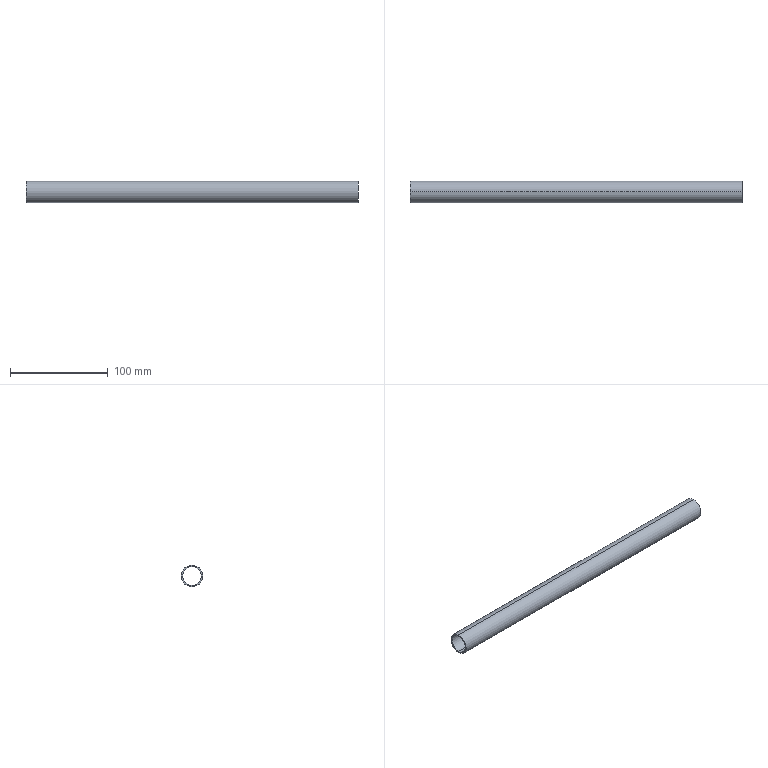Part | STEP file | copper tube 20_default_machined_ | 1 solid | 6 faces | box 340 x 22 x 22 mm | volume 32845 mm3 | cylinder 4 | plane 2 | commonest cylinder face diameters 19 x2 22 x2
STEP:
#1=CARTESIAN_POINT('',(0.,0.,0.));
#2=DIRECTION('',(0.,0.,1.));
#3=DIRECTION('',(1.,0.,0.));
#4=AXIS2_PLACEMENT_3D('',#1,#2,#3);
#5=CARTESIAN_POINT('',(340.,0.,11.));
#6=VERTEX_POINT('',#5);
#7=CARTESIAN_POINT('',(340.,0.,-11.));
#8=VERTEX_POINT('',#7);
#9=CARTESIAN_POINT('',(340.,0.,0.));
#10=DIRECTION('',(-1.,0.,0.));
#11=DIRECTION('',(0.,0.,1.));
#12=AXIS2_PLACEMENT_3D('',#9,#10,#11);
#13=CIRCLE('',#12,11.);
#14=CARTESIAN_POINT('',(340.,0.,0.));
#15=DIRECTION('',(-1.,0.,0.));
#16=DIRECTION('',(0.,0.,1.));
#17=AXIS2_PLACEMENT_3D('',#14,#15,#16);
#18=CYLINDRICAL_SURFACE('',#17,11.);
#19=CARTESIAN_POINT('',(0.,0.));
#20=DIRECTION('',(1.,0.));
#21=VECTOR('',#20,1.);
#22=LINE('',#19,#21);
#23=(GEOMETRIC_REPRESENTATION_CONTEXT(2)PARAMETRIC_REPRESENTATION_CONTEXT()REPRESENTATION_CONTEXT('',''));
#24=DEFINITIONAL_REPRESENTATION('',(#22),#23);
#25=PCURVE('',#18,#24);
#26=CARTESIAN_POINT('',(340.,0.,0.));
#27=DIRECTION('',(1.,0.,0.));
#28=DIRECTION('',(0.,0.,-1.));
#29=AXIS2_PLACEMENT_3D('',#26,#27,#28);
#30=PLANE('',#29);
#31=CARTESIAN_POINT('',(-11.,0.));
#32=CARTESIAN_POINT('',(-11.,19.053));
#33=CARTESIAN_POINT('',(5.5,9.526));
#34=CARTESIAN_POINT('',(22.,0.));
#35=CARTESIAN_POINT('',(5.5,-9.526));
#36=CARTESIAN_POINT('',(-11.,-19.053));
#37=CARTESIAN_POINT('',(-11.,0.));
#38=(BOUNDED_CURVE()B_SPLINE_CURVE(2,(#31,#32,#33,#34,#35,#36,#37),.UNSPECIFIED.,.T.,.F.)B_SPLINE_CURVE_WITH_KNOTS((1,2,2,2,2,1),(-2.094,0.,2.094,4.189,6.283,8.378),.UNSPECIFIED.)CURVE()GEOMETRIC_REPRESENTATION_ITEM()RATIONAL_B_SPLINE_CURVE((1.,0.5,1.,0.5,1.,0.5,1.))REPRESENTATION_ITEM(''));
#39=(GEOMETRIC_REPRESENTATION_CONTEXT(2)PARAMETRIC_REPRESENTATION_CONTEXT()REPRESENTATION_CONTEXT('',''));
#40=DEFINITIONAL_REPRESENTATION('',(#38),#39);
#41=PCURVE('',#30,#40);
#42=SURFACE_CURVE('',#13,(#25,#41),.PCURVE_S1.);
#43=EDGE_CURVE('',#6,#8,#42,.T.);
#44=ORIENTED_EDGE('',*,*,#43,.T.);
#45=CARTESIAN_POINT('',(0.,0.,-11.));
#46=VERTEX_POINT('',#45);
#47=CARTESIAN_POINT('',(340.,0.,-11.));
#48=DIRECTION('',(-1.,0.,0.));
#49=VECTOR('',#48,1.);
#50=LINE('',#47,#49);
#51=CARTESIAN_POINT('',(3.142,0.));
#52=DIRECTION('',(0.,1.));
#53=VECTOR('',#52,1.);
#54=LINE('',#51,#53);
#55=(GEOMETRIC_REPRESENTATION_CONTEXT(2)PARAMETRIC_REPRESENTATION_CONTEXT()REPRESENTATION_CONTEXT('',''));
#56=DEFINITIONAL_REPRESENTATION('',(#54),#55);
#57=PCURVE('',#18,#56);
#58=CARTESIAN_POINT('',(340.,0.,0.));
#59=DIRECTION('',(-1.,0.,0.));
#60=DIRECTION('',(0.,0.,1.));
#61=AXIS2_PLACEMENT_3D('',#58,#59,#60);
#62=CYLINDRICAL_SURFACE('',#61,11.);
#63=CARTESIAN_POINT('',(3.142,0.));
#64=DIRECTION('',(0.,1.));
#65=VECTOR('',#64,1.);
#66=LINE('',#63,#65);
#67=(GEOMETRIC_REPRESENTATION_CONTEXT(2)PARAMETRIC_REPRESENTATION_CONTEXT()REPRESENTATION_CONTEXT('',''));
#68=DEFINITIONAL_REPRESENTATION('',(#66),#67);
#69=PCURVE('',#62,#68);
#70=SURFACE_CURVE('',#50,(#57,#69),.PCURVE_S1.);
#71=EDGE_CURVE('',#8,#46,#70,.T.);
#72=ORIENTED_EDGE('',*,*,#71,.T.);
#73=CARTESIAN_POINT('',(0.,0.,11.));
#74=VERTEX_POINT('',#73);
#75=CARTESIAN_POINT('',(0.,0.,0.));
#76=DIRECTION('',(1.,0.,0.));
#77=DIRECTION('',(0.,0.,1.));
#78=AXIS2_PLACEMENT_3D('',#75,#76,#77);
#79=CIRCLE('',#78,11.);
#80=CARTESIAN_POINT('',(6.283,340.));
#81=DIRECTION('',(-1.,0.));
#82=VECTOR('',#81,1.);
#83=LINE('',#80,#82);
#84=(GEOMETRIC_REPRESENTATION_CONTEXT(2)PARAMETRIC_REPRESENTATION_CONTEXT()REPRESENTATION_CONTEXT('',''));
#85=DEFINITIONAL_REPRESENTATION('',(#83),#84);
#86=PCURVE('',#18,#85);
#87=CARTESIAN_POINT('',(0.,0.,0.));
#88=DIRECTION('',(1.,0.,0.));
#89=DIRECTION('',(0.,0.,-1.));
#90=AXIS2_PLACEMENT_3D('',#87,#88,#89);
#91=PLANE('',#90);
#92=CARTESIAN_POINT('',(0.,0.));
#93=DIRECTION('',(-1.,0.));
#94=AXIS2_PLACEMENT_2D('',#92,#93);
#95=CIRCLE('',#94,11.);
#96=(GEOMETRIC_REPRESENTATION_CONTEXT(2)PARAMETRIC_REPRESENTATION_CONTEXT()REPRESENTATION_CONTEXT('',''));
#97=DEFINITIONAL_REPRESENTATION('',(#95),#96);
#98=PCURVE('',#91,#97);
#99=SURFACE_CURVE('',#79,(#86,#98),.PCURVE_S1.);
#100=EDGE_CURVE('',#46,#74,#99,.T.);
#101=ORIENTED_EDGE('',*,*,#100,.T.);
#102=CARTESIAN_POINT('',(340.,0.,11.));
#103=DIRECTION('',(-1.,0.,0.));
#104=VECTOR('',#103,1.);
#105=LINE('',#102,#104);
#106=CARTESIAN_POINT('',(0.,0.));
#107=DIRECTION('',(0.,1.));
#108=VECTOR('',#107,1.);
#109=LINE('',#106,#108);
#110=(GEOMETRIC_REPRESENTATION_CONTEXT(2)PARAMETRIC_REPRESENTATION_CONTEXT()REPRESENTATION_CONTEXT('',''));
#111=DEFINITIONAL_REPRESENTATION('',(#109),#110);
#112=PCURVE('',#18,#111);
#113=CARTESIAN_POINT('',(6.283,0.));
#114=DIRECTION('',(0.,1.));
#115=VECTOR('',#114,1.);
#116=LINE('',#113,#115);
#117=(GEOMETRIC_REPRESENTATION_CONTEXT(2)PARAMETRIC_REPRESENTATION_CONTEXT()REPRESENTATION_CONTEXT('',''));
#118=DEFINITIONAL_REPRESENTATION('',(#116),#117);
#119=PCURVE('',#62,#118);
#120=SURFACE_CURVE('',#105,(#112,#119),.PCURVE_S1.);
#121=EDGE_CURVE('',#6,#74,#120,.T.);
#122=ORIENTED_EDGE('',*,*,#121,.F.);
#123=EDGE_LOOP('',(#44,#72,#101,#122));
#124=FACE_BOUND('',#123,.T.);
#125=ADVANCED_FACE('',(#124),#18,.T.);
#126=CARTESIAN_POINT('',(340.,0.,9.5));
#127=VERTEX_POINT('',#126);
#128=CARTESIAN_POINT('',(0.,0.,9.5));
#129=VERTEX_POINT('',#128);
#130=CARTESIAN_POINT('',(340.,0.,9.5));
#131=DIRECTION('',(-1.,0.,0.));
#132=VECTOR('',#131,1.);
#133=LINE('',#130,#132);
#134=CARTESIAN_POINT('',(340.,0.,0.));
#135=DIRECTION('',(-1.,0.,0.));
#136=DIRECTION('',(0.,0.,1.));
#137=AXIS2_PLACEMENT_3D('',#134,#135,#136);
#138=CYLINDRICAL_SURFACE('',#137,9.5);
#139=CARTESIAN_POINT('',(6.283,0.));
#140=DIRECTION('',(0.,1.));
#141=VECTOR('',#140,1.);
#142=LINE('',#139,#141);
#143=(GEOMETRIC_REPRESENTATION_CONTEXT(2)PARAMETRIC_REPRESENTATION_CONTEXT()REPRESENTATION_CONTEXT('',''));
#144=DEFINITIONAL_REPRESENTATION('',(#142),#143);
#145=PCURVE('',#138,#144);
#146=CARTESIAN_POINT('',(340.,0.,0.));
#147=DIRECTION('',(-1.,0.,0.));
#148=DIRECTION('',(0.,0.,1.));
#149=AXIS2_PLACEMENT_3D('',#146,#147,#148);
#150=CYLINDRICAL_SURFACE('',#149,9.5);
#151=CARTESIAN_POINT('',(0.,0.));
#152=DIRECTION('',(0.,1.));
#153=VECTOR('',#152,1.);
#154=LINE('',#151,#153);
#155=(GEOMETRIC_REPRESENTATION_CONTEXT(2)PARAMETRIC_REPRESENTATION_CONTEXT()REPRESENTATION_CONTEXT('',''));
#156=DEFINITIONAL_REPRESENTATION('',(#154),#155);
#157=PCURVE('',#150,#156);
#158=SURFACE_CURVE('',#133,(#145,#157),.PCURVE_S1.);
#159=EDGE_CURVE('',#127,#129,#158,.T.);
#160=ORIENTED_EDGE('',*,*,#159,.T.);
#161=CARTESIAN_POINT('',(0.,0.,-9.5));
#162=VERTEX_POINT('',#161);
#163=CARTESIAN_POINT('',(0.,0.,0.));
#164=DIRECTION('',(-1.,0.,0.));
#165=DIRECTION('',(0.,0.,1.));
#166=AXIS2_PLACEMENT_3D('',#163,#164,#165);
#167=CIRCLE('',#166,9.5);
#168=CARTESIAN_POINT('',(0.,340.));
#169=DIRECTION('',(1.,0.));
#170=VECTOR('',#169,1.);
#171=LINE('',#168,#170);
#172=(GEOMETRIC_REPRESENTATION_CONTEXT(2)PARAMETRIC_REPRESENTATION_CONTEXT()REPRESENTATION_CONTEXT('',''));
#173=DEFINITIONAL_REPRESENTATION('',(#171),#172);
#174=PCURVE('',#138,#173);
#175=CARTESIAN_POINT('',(-9.5,0.));
#176=CARTESIAN_POINT('',(-9.5,16.454));
#177=CARTESIAN_POINT('',(4.75,8.227));
#178=CARTESIAN_POINT('',(19.,0.));
#179=CARTESIAN_POINT('',(4.75,-8.227));
#180=CARTESIAN_POINT('',(-9.5,-16.454));
#181=CARTESIAN_POINT('',(-9.5,0.));
#182=(BOUNDED_CURVE()B_SPLINE_CURVE(2,(#175,#176,#177,#178,#179,#180,#181),.UNSPECIFIED.,.T.,.F.)B_SPLINE_CURVE_WITH_KNOTS((1,2,2,2,2,1),(-2.094,0.,2.094,4.189,6.283,8.378),.UNSPECIFIED.)CURVE()GEOMETRIC_REPRESENTATION_ITEM()RATIONAL_B_SPLINE_CURVE((1.,0.5,1.,0.5,1.,0.5,1.))REPRESENTATION_ITEM(''));
#183=(GEOMETRIC_REPRESENTATION_CONTEXT(2)PARAMETRIC_REPRESENTATION_CONTEXT()REPRESENTATION_CONTEXT('',''));
#184=DEFINITIONAL_REPRESENTATION('',(#182),#183);
#185=PCURVE('',#91,#184);
#186=SURFACE_CURVE('',#167,(#174,#185),.PCURVE_S1.);
#187=EDGE_CURVE('',#162,#129,#186,.T.);
#188=ORIENTED_EDGE('',*,*,#187,.F.);
#189=CARTESIAN_POINT('',(340.,0.,-9.5));
#190=VERTEX_POINT('',#189);
#191=CARTESIAN_POINT('',(340.,0.,-9.5));
#192=DIRECTION('',(-1.,0.,0.));
#193=VECTOR('',#192,1.);
#194=LINE('',#191,#193);
#195=CARTESIAN_POINT('',(3.142,0.));
#196=DIRECTION('',(0.,1.));
#197=VECTOR('',#196,1.);
#198=LINE('',#195,#197);
#199=(GEOMETRIC_REPRESENTATION_CONTEXT(2)PARAMETRIC_REPRESENTATION_CONTEXT()REPRESENTATION_CONTEXT('',''));
#200=DEFINITIONAL_REPRESENTATION('',(#198),#199);
#201=PCURVE('',#138,#200);
#202=CARTESIAN_POINT('',(3.142,0.));
#203=DIRECTION('',(0.,1.));
#204=VECTOR('',#203,1.);
#205=LINE('',#202,#204);
#206=(GEOMETRIC_REPRESENTATION_CONTEXT(2)PARAMETRIC_REPRESENTATION_CONTEXT()REPRESENTATION_CONTEXT('',''));
#207=DEFINITIONAL_REPRESENTATION('',(#205),#206);
#208=PCURVE('',#150,#207);
#209=SURFACE_CURVE('',#194,(#201,#208),.PCURVE_S1.);
#210=EDGE_CURVE('',#190,#162,#209,.T.);
#211=ORIENTED_EDGE('',*,*,#210,.F.);
#212=CARTESIAN_POINT('',(340.,0.,0.));
#213=DIRECTION('',(-1.,0.,0.));
#214=DIRECTION('',(0.,0.,1.));
#215=AXIS2_PLACEMENT_3D('',#212,#213,#214);
#216=CIRCLE('',#215,9.5);
#217=CARTESIAN_POINT('',(0.,0.));
#218=DIRECTION('',(1.,0.));
#219=VECTOR('',#218,1.);
#220=LINE('',#217,#219);
#221=(GEOMETRIC_REPRESENTATION_CONTEXT(2)PARAMETRIC_REPRESENTATION_CONTEXT()REPRESENTATION_CONTEXT('',''));
#222=DEFINITIONAL_REPRESENTATION('',(#220),#221);
#223=PCURVE('',#138,#222);
#224=CARTESIAN_POINT('',(-9.5,0.));
#225=CARTESIAN_POINT('',(-9.5,16.454));
#226=CARTESIAN_POINT('',(4.75,8.227));
#227=CARTESIAN_POINT('',(19.,0.));
#228=CARTESIAN_POINT('',(4.75,-8.227));
#229=CARTESIAN_POINT('',(-9.5,-16.454));
#230=CARTESIAN_POINT('',(-9.5,0.));
#231=(BOUNDED_CURVE()B_SPLINE_CURVE(2,(#224,#225,#226,#227,#228,#229,#230),.UNSPECIFIED.,.T.,.F.)B_SPLINE_CURVE_WITH_KNOTS((1,2,2,2,2,1),(-2.094,0.,2.094,4.189,6.283,8.378),.UNSPECIFIED.)CURVE()GEOMETRIC_REPRESENTATION_ITEM()RATIONAL_B_SPLINE_CURVE((1.,0.5,1.,0.5,1.,0.5,1.))REPRESENTATION_ITEM(''));
#232=(GEOMETRIC_REPRESENTATION_CONTEXT(2)PARAMETRIC_REPRESENTATION_CONTEXT()REPRESENTATION_CONTEXT('',''));
#233=DEFINITIONAL_REPRESENTATION('',(#231),#232);
#234=PCURVE('',#30,#233);
#235=SURFACE_CURVE('',#216,(#223,#234),.PCURVE_S1.);
#236=EDGE_CURVE('',#190,#127,#235,.T.);
#237=ORIENTED_EDGE('',*,*,#236,.T.);
#238=EDGE_LOOP('',(#160,#188,#211,#237));
#239=FACE_BOUND('',#238,.F.);
#240=ADVANCED_FACE('',(#239),#138,.F.);
#241=ORIENTED_EDGE('',*,*,#71,.F.);
#242=CARTESIAN_POINT('',(340.,0.,0.));
#243=DIRECTION('',(-1.,0.,0.));
#244=DIRECTION('',(0.,0.,1.));
#245=AXIS2_PLACEMENT_3D('',#242,#243,#244);
#246=CIRCLE('',#245,11.);
#247=CARTESIAN_POINT('',(0.,0.));
#248=DIRECTION('',(1.,0.));
#249=VECTOR('',#248,1.);
#250=LINE('',#247,#249);
#251=(GEOMETRIC_REPRESENTATION_CONTEXT(2)PARAMETRIC_REPRESENTATION_CONTEXT()REPRESENTATION_CONTEXT('',''));
#252=DEFINITIONAL_REPRESENTATION('',(#250),#251);
#253=PCURVE('',#62,#252);
#254=CARTESIAN_POINT('',(-11.,0.));
#255=CARTESIAN_POINT('',(-11.,19.053));
#256=CARTESIAN_POINT('',(5.5,9.526));
#257=CARTESIAN_POINT('',(22.,0.));
#258=CARTESIAN_POINT('',(5.5,-9.526));
#259=CARTESIAN_POINT('',(-11.,-19.053));
#260=CARTESIAN_POINT('',(-11.,0.));
#261=(BOUNDED_CURVE()B_SPLINE_CURVE(2,(#254,#255,#256,#257,#258,#259,#260),.UNSPECIFIED.,.T.,.F.)B_SPLINE_CURVE_WITH_KNOTS((1,2,2,2,2,1),(-2.094,0.,2.094,4.189,6.283,8.378),.UNSPECIFIED.)CURVE()GEOMETRIC_REPRESENTATION_ITEM()RATIONAL_B_SPLINE_CURVE((1.,0.5,1.,0.5,1.,0.5,1.))REPRESENTATION_ITEM(''));
#262=(GEOMETRIC_REPRESENTATION_CONTEXT(2)PARAMETRIC_REPRESENTATION_CONTEXT()REPRESENTATION_CONTEXT('',''));
#263=DEFINITIONAL_REPRESENTATION('',(#261),#262);
#264=PCURVE('',#30,#263);
#265=SURFACE_CURVE('',#246,(#253,#264),.PCURVE_S1.);
#266=EDGE_CURVE('',#8,#6,#265,.T.);
#267=ORIENTED_EDGE('',*,*,#266,.T.);
#268=ORIENTED_EDGE('',*,*,#121,.T.);
#269=CARTESIAN_POINT('',(0.,0.,0.));
#270=DIRECTION('',(1.,0.,0.));
#271=DIRECTION('',(0.,0.,1.));
#272=AXIS2_PLACEMENT_3D('',#269,#270,#271);
#273=CIRCLE('',#272,11.);
#274=CARTESIAN_POINT('',(6.283,340.));
#275=DIRECTION('',(-1.,0.));
#276=VECTOR('',#275,1.);
#277=LINE('',#274,#276);
#278=(GEOMETRIC_REPRESENTATION_CONTEXT(2)PARAMETRIC_REPRESENTATION_CONTEXT()REPRESENTATION_CONTEXT('',''));
#279=DEFINITIONAL_REPRESENTATION('',(#277),#278);
#280=PCURVE('',#62,#279);
#281=CARTESIAN_POINT('',(0.,0.));
#282=DIRECTION('',(-1.,0.));
#283=AXIS2_PLACEMENT_2D('',#281,#282);
#284=CIRCLE('',#283,11.);
#285=(GEOMETRIC_REPRESENTATION_CONTEXT(2)PARAMETRIC_REPRESENTATION_CONTEXT()REPRESENTATION_CONTEXT('',''));
#286=DEFINITIONAL_REPRESENTATION('',(#284),#285);
#287=PCURVE('',#91,#286);
#288=SURFACE_CURVE('',#273,(#280,#287),.PCURVE_S1.);
#289=EDGE_CURVE('',#74,#46,#288,.T.);
#290=ORIENTED_EDGE('',*,*,#289,.T.);
#291=EDGE_LOOP('',(#241,#267,#268,#290));
#292=FACE_BOUND('',#291,.T.);
#293=ADVANCED_FACE('',(#292),#62,.T.);
#294=ORIENTED_EDGE('',*,*,#289,.F.);
#295=ORIENTED_EDGE('',*,*,#100,.F.);
#296=EDGE_LOOP('',(#294,#295));
#297=FACE_BOUND('',#296,.T.);
#298=CARTESIAN_POINT('',(0.,0.,0.));
#299=DIRECTION('',(-1.,0.,0.));
#300=DIRECTION('',(0.,0.,1.));
#301=AXIS2_PLACEMENT_3D('',#298,#299,#300);
#302=CIRCLE('',#301,9.5);
#303=CARTESIAN_POINT('',(-9.5,0.));
#304=CARTESIAN_POINT('',(-9.5,16.454));
#305=CARTESIAN_POINT('',(4.75,8.227));
#306=CARTESIAN_POINT('',(19.,0.));
#307=CARTESIAN_POINT('',(4.75,-8.227));
#308=CARTESIAN_POINT('',(-9.5,-16.454));
#309=CARTESIAN_POINT('',(-9.5,0.));
#310=(BOUNDED_CURVE()B_SPLINE_CURVE(2,(#303,#304,#305,#306,#307,#308,#309),.UNSPECIFIED.,.T.,.F.)B_SPLINE_CURVE_WITH_KNOTS((1,2,2,2,2,1),(-2.094,0.,2.094,4.189,6.283,8.378),.UNSPECIFIED.)CURVE()GEOMETRIC_REPRESENTATION_ITEM()RATIONAL_B_SPLINE_CURVE((1.,0.5,1.,0.5,1.,0.5,1.))REPRESENTATION_ITEM(''));
#311=(GEOMETRIC_REPRESENTATION_CONTEXT(2)PARAMETRIC_REPRESENTATION_CONTEXT()REPRESENTATION_CONTEXT('',''));
#312=DEFINITIONAL_REPRESENTATION('',(#310),#311);
#313=PCURVE('',#91,#312);
#314=CARTESIAN_POINT('',(0.,340.));
#315=DIRECTION('',(1.,0.));
#316=VECTOR('',#315,1.);
#317=LINE('',#314,#316);
#318=(GEOMETRIC_REPRESENTATION_CONTEXT(2)PARAMETRIC_REPRESENTATION_CONTEXT()REPRESENTATION_CONTEXT('',''));
#319=DEFINITIONAL_REPRESENTATION('',(#317),#318);
#320=PCURVE('',#150,#319);
#321=SURFACE_CURVE('',#302,(#313,#320),.PCURVE_S1.);
#322=EDGE_CURVE('',#129,#162,#321,.T.);
#323=ORIENTED_EDGE('',*,*,#322,.F.);
#324=ORIENTED_EDGE('',*,*,#187,.F.);
#325=EDGE_LOOP('',(#323,#324));
#326=FACE_BOUND('',#325,.T.);
#327=ADVANCED_FACE('',(#297,#326),#91,.F.);
#328=ORIENTED_EDGE('',*,*,#43,.F.);
#329=ORIENTED_EDGE('',*,*,#266,.F.);
#330=EDGE_LOOP('',(#328,#329));
#331=FACE_BOUND('',#330,.T.);
#332=CARTESIAN_POINT('',(340.,0.,0.));
#333=DIRECTION('',(-1.,0.,0.));
#334=DIRECTION('',(0.,0.,1.));
#335=AXIS2_PLACEMENT_3D('',#332,#333,#334);
#336=CIRCLE('',#335,9.5);
#337=CARTESIAN_POINT('',(-9.5,0.));
#338=CARTESIAN_POINT('',(-9.5,16.454));
#339=CARTESIAN_POINT('',(4.75,8.227));
#340=CARTESIAN_POINT('',(19.,0.));
#341=CARTESIAN_POINT('',(4.75,-8.227));
#342=CARTESIAN_POINT('',(-9.5,-16.454));
#343=CARTESIAN_POINT('',(-9.5,0.));
#344=(BOUNDED_CURVE()B_SPLINE_CURVE(2,(#337,#338,#339,#340,#341,#342,#343),.UNSPECIFIED.,.T.,.F.)B_SPLINE_CURVE_WITH_KNOTS((1,2,2,2,2,1),(-2.094,0.,2.094,4.189,6.283,8.378),.UNSPECIFIED.)CURVE()GEOMETRIC_REPRESENTATION_ITEM()RATIONAL_B_SPLINE_CURVE((1.,0.5,1.,0.5,1.,0.5,1.))REPRESENTATION_ITEM(''));
#345=(GEOMETRIC_REPRESENTATION_CONTEXT(2)PARAMETRIC_REPRESENTATION_CONTEXT()REPRESENTATION_CONTEXT('',''));
#346=DEFINITIONAL_REPRESENTATION('',(#344),#345);
#347=PCURVE('',#30,#346);
#348=CARTESIAN_POINT('',(0.,0.));
#349=DIRECTION('',(1.,0.));
#350=VECTOR('',#349,1.);
#351=LINE('',#348,#350);
#352=(GEOMETRIC_REPRESENTATION_CONTEXT(2)PARAMETRIC_REPRESENTATION_CONTEXT()REPRESENTATION_CONTEXT('',''));
#353=DEFINITIONAL_REPRESENTATION('',(#351),#352);
#354=PCURVE('',#150,#353);
#355=SURFACE_CURVE('',#336,(#347,#354),.PCURVE_S1.);
#356=EDGE_CURVE('',#127,#190,#355,.T.);
#357=ORIENTED_EDGE('',*,*,#356,.T.);
#358=ORIENTED_EDGE('',*,*,#236,.T.);
#359=EDGE_LOOP('',(#357,#358));
#360=FACE_BOUND('',#359,.T.);
#361=ADVANCED_FACE('',(#331,#360),#30,.T.);
#362=ORIENTED_EDGE('',*,*,#322,.F.);
#363=ORIENTED_EDGE('',*,*,#159,.F.);
#364=ORIENTED_EDGE('',*,*,#356,.T.);
#365=ORIENTED_EDGE('',*,*,#210,.T.);
#366=EDGE_LOOP('',(#362,#363,#364,#365));
#367=FACE_BOUND('',#366,.F.);
#368=ADVANCED_FACE('',(#367),#150,.F.);
#369=CLOSED_SHELL('',(#125,#240,#293,#327,#361,#368));
#370=MANIFOLD_SOLID_BREP('',#369);
#371=(LENGTH_UNIT()NAMED_UNIT(*)SI_UNIT(.MILLI.,.METRE.));
#372=UNCERTAINTY_MEASURE_WITH_UNIT(LENGTH_MEASURE(0.0000001),#371,'','');
#373=(NAMED_UNIT(*)PLANE_ANGLE_UNIT()SI_UNIT($,.RADIAN.));
#374=(NAMED_UNIT(*)SI_UNIT($,.STERADIAN.)SOLID_ANGLE_UNIT());
#375=(GEOMETRIC_REPRESENTATION_CONTEXT(3)GLOBAL_UNCERTAINTY_ASSIGNED_CONTEXT((#372))GLOBAL_UNIT_ASSIGNED_CONTEXT((#371,#373,#374))REPRESENTATION_CONTEXT('',''));
#376=ADVANCED_BREP_SHAPE_REPRESENTATION('',(#4,#370),#375);